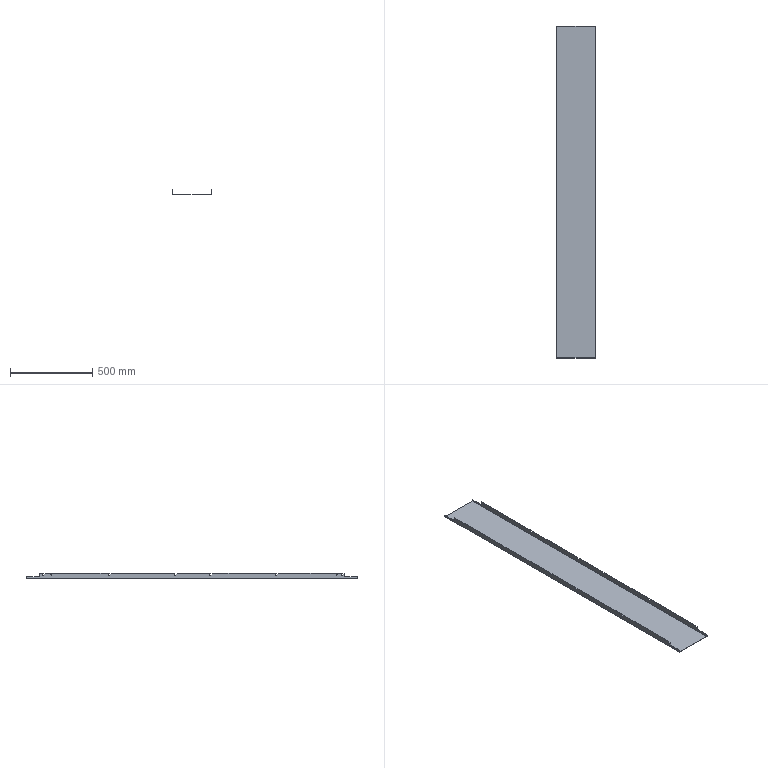Part | 1 solid | 102 faces | box 235 x 2016 x 33 mm | volume 710517 mm3 | plane 66 | cylinder 36 | commonest cylinder face diameters 8.2 x24 6 x8 0.4 x2 2.8 x2